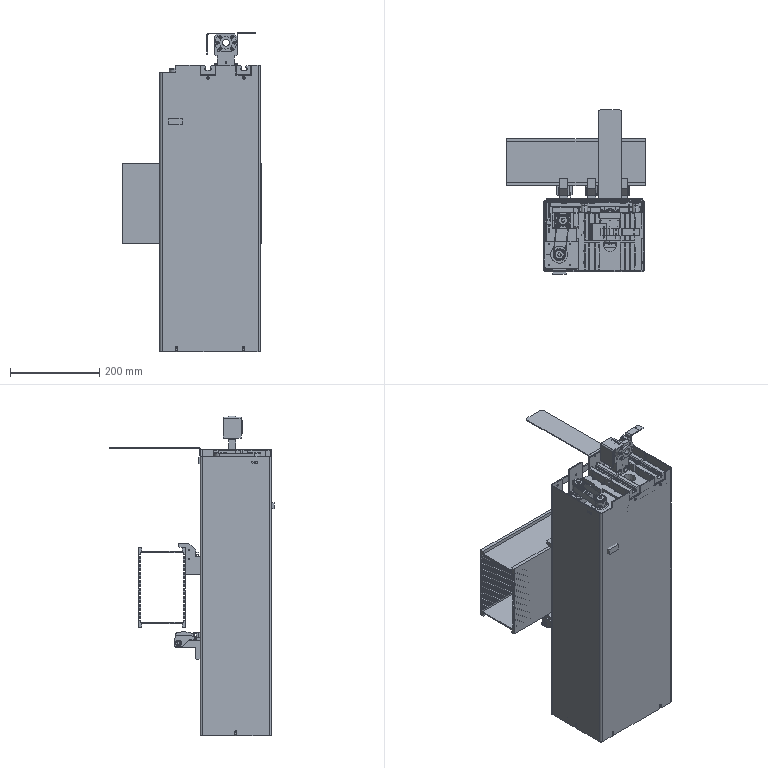Part | NX | features BREP 73 | 118 solids | 8389 faces | volume 4800109 mm3 | plane 3857 | cylinder 3340 | cone 604 | torus 244 | spline 218 | sphere 126 | commonest cylinder face diameters 25 x371 2.5 x296 10 x221 6 x198 3.3 x174 12 x165